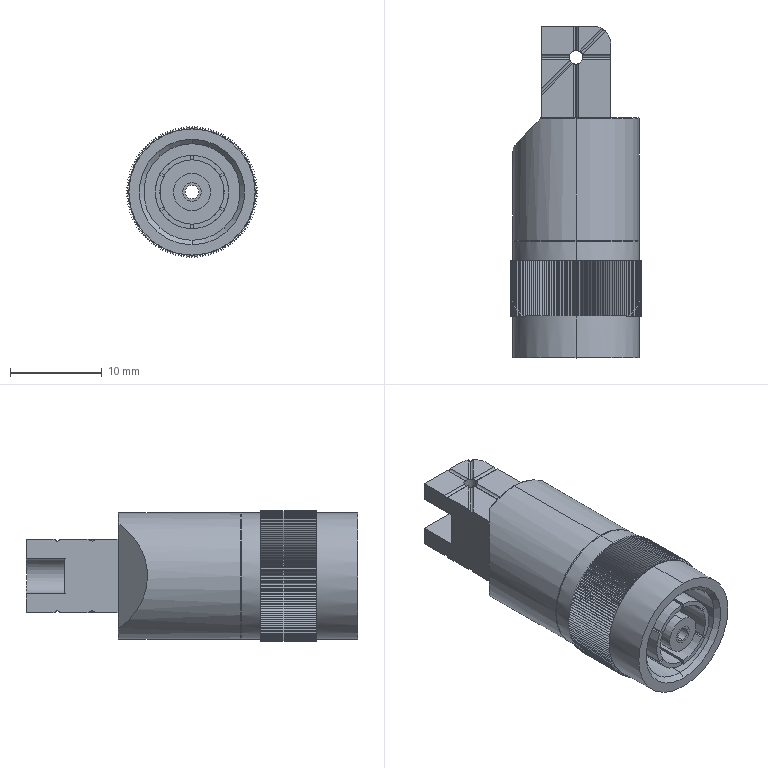Part | SolidWorks | 5 solids | 771 faces | box 14.217 x 36.1 x 14.22 mm | volume 3487 mm3 | plane 678 | cylinder 74 | torus 9 | spline 8 | cone 2 | commonest cylinder face diameters 0.51 x24 10 x14 1.5 x6 2 x4 7 x4 10.5 x4